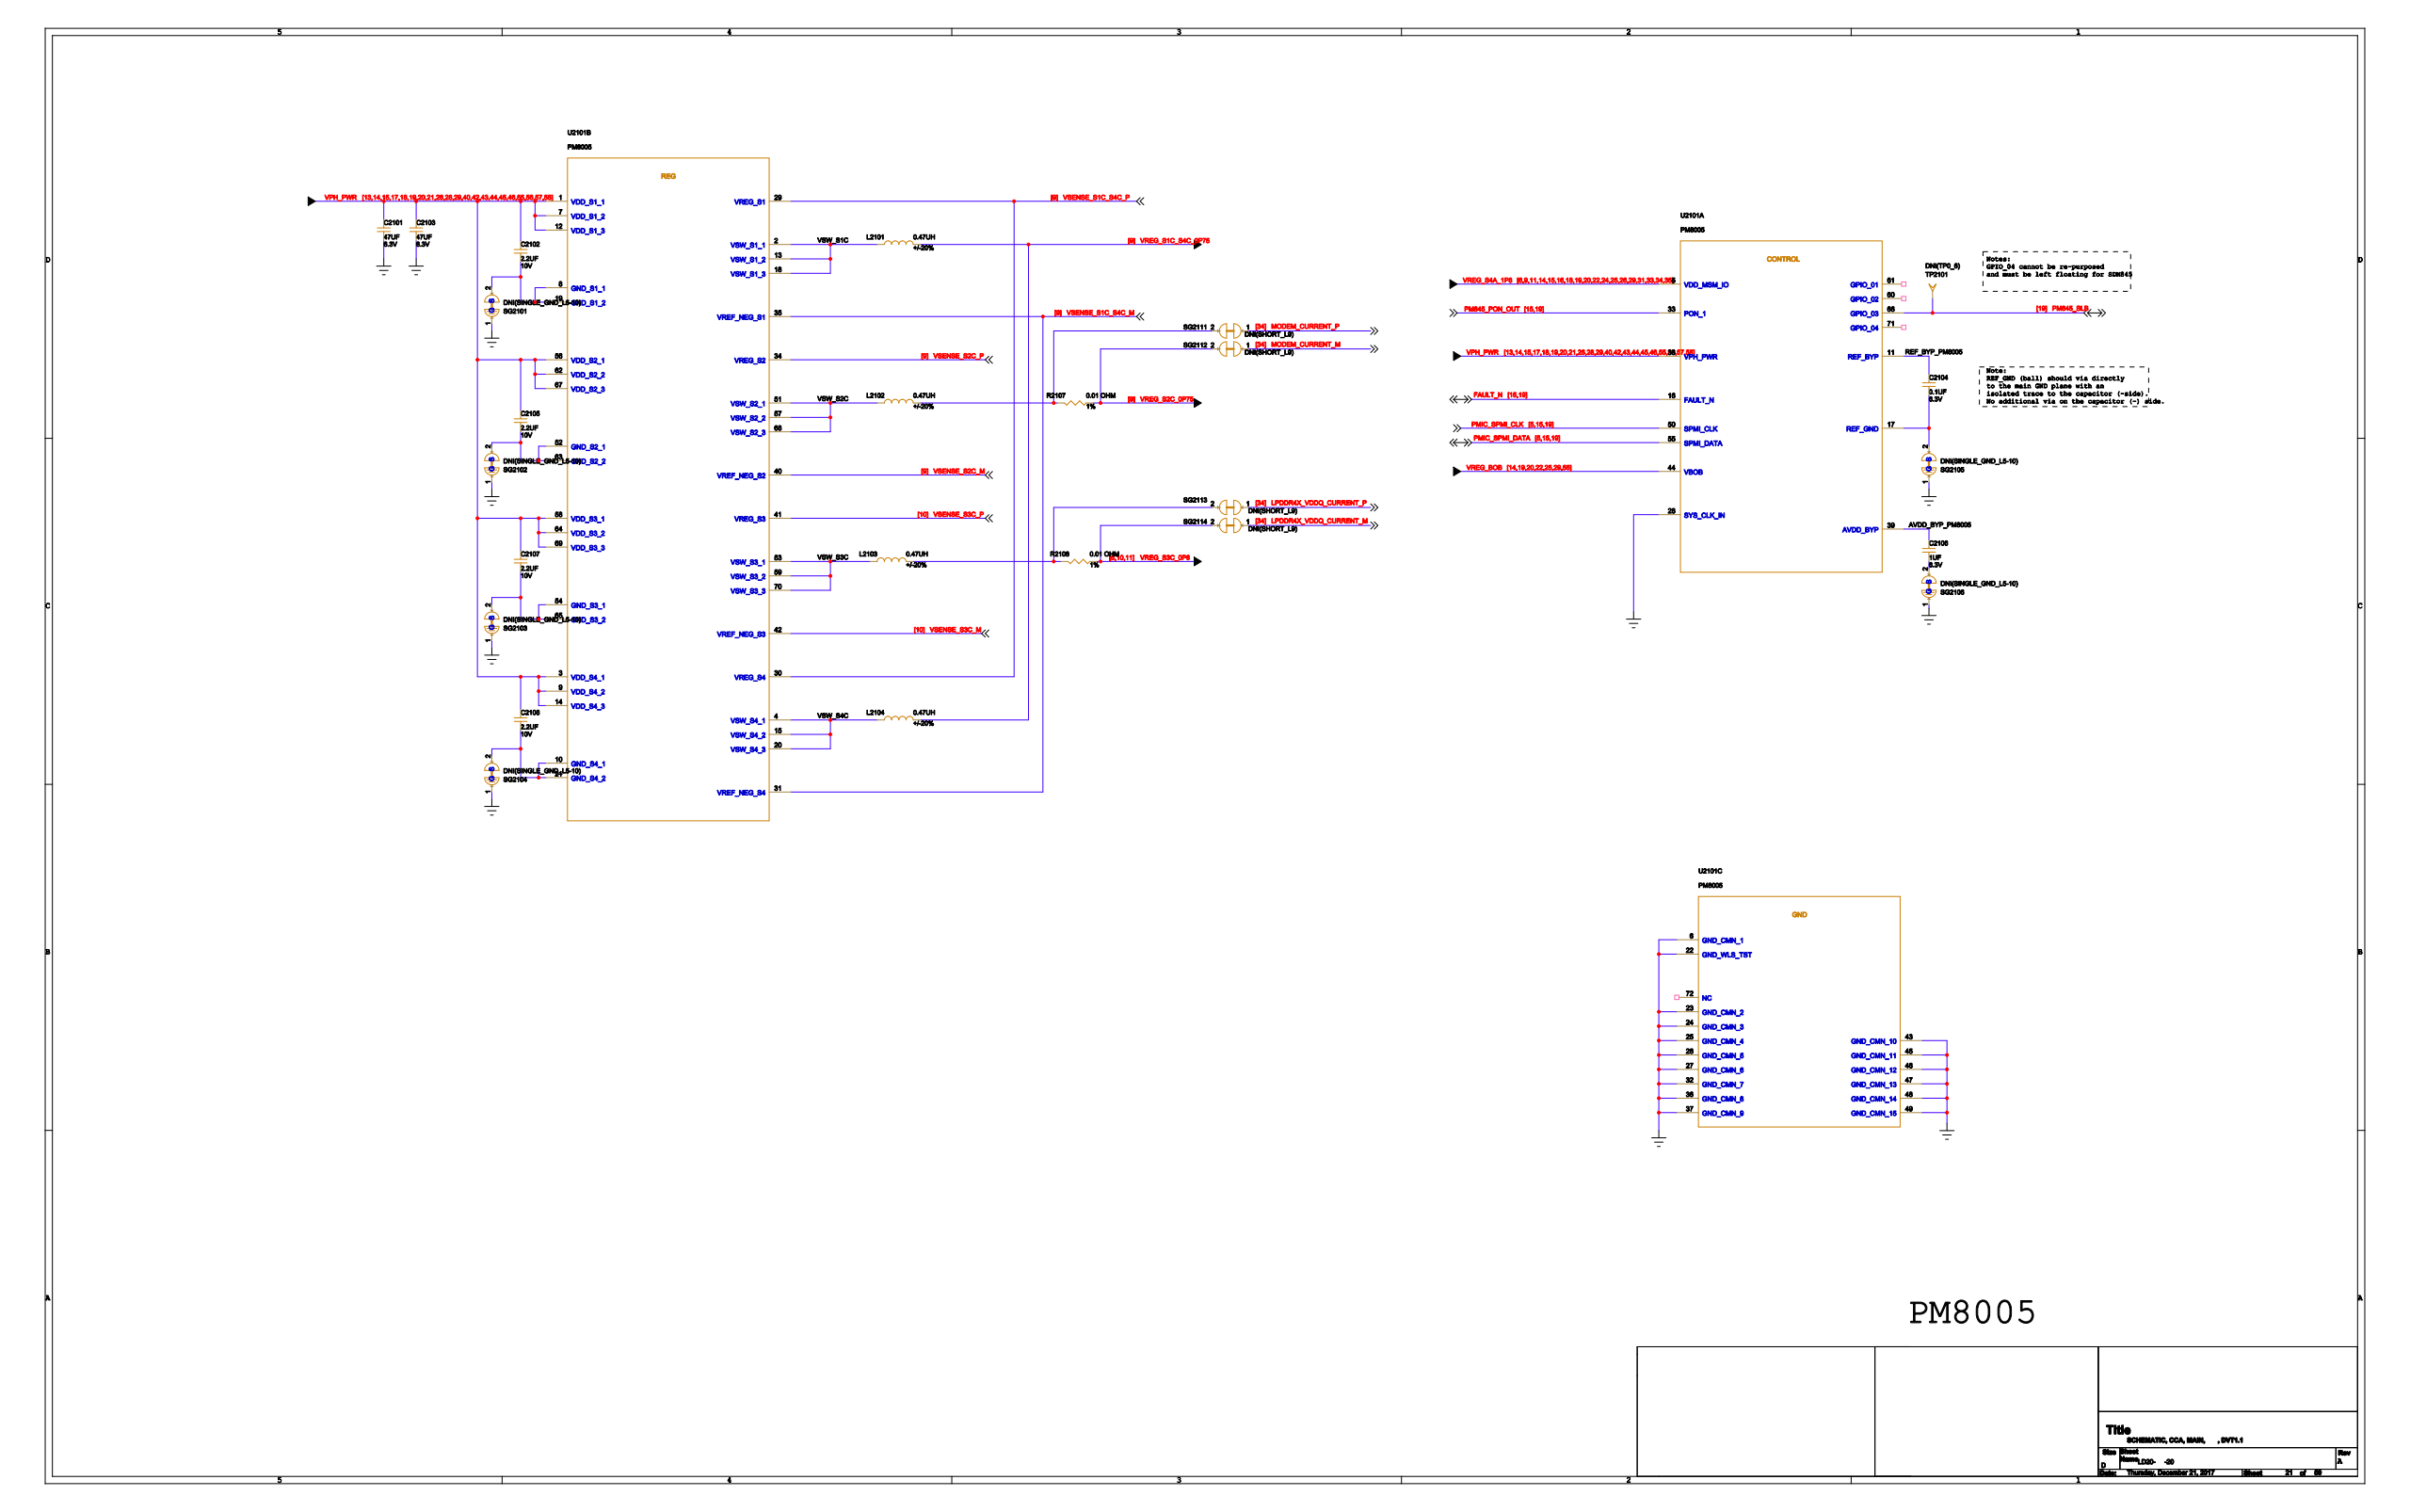Circuit board | Cadence Allegro | 1520 parts | 1149 nets | one sheet of the schematic
Parts on this sheet (reference | value | footprint):
C2101 | 47UF | 2P0603R
C2102 | 2.2UF | 2P0201R
C2103 | 47UF | 2P0603R
C2104 | 0.1UF | 2P0201R
C2105 | 2.2UF | 2P0201R
C2106 | 1UF | 2P0201R
C2107 | 2.2UF | 2P0201R
C2108 | 2.2UF | 2P0201R
L2101 | 0.47UH | 2PSM87X71NV2
L2102 | 0.47UH | 2PSM87X71NV2
L2103 | 0.47UH | 2PSM87X71NV2
L2104 | 0.47UH | 2PSM87X71NV2
R2107 | 0.01 OHM | 2P0603R
R2108 | 0.01 OHM | 2P0603R
SG2101 | DNI(SINGLE_GND_L5-10) | GND_L5-10
SG2102 | DNI(SINGLE_GND_L5-10) | GND_L5-10
SG2103 | DNI(SINGLE_GND_L5-10) | GND_L5-10
SG2104 | DNI(SINGLE_GND_L5-10) | GND_L5-10
SG2105 | DNI(SINGLE_GND_L5-10) | GND_L5-10
SG2106 | DNI(SINGLE_GND_L5-10) | GND_L5-10
SG2111 | DNI(SHORT_L9) | SHORT_L9_2REC08X12
SG2112 | DNI(SHORT_L9) | SHORT_L9_2REC08X12
SG2113 | DNI(SHORT_L9) | SHORT_L9_2REC08X12
SG2114 | DNI(SHORT_L9) | SHORT_L9_2REC08X12
TP2101 | DNI(TP0_6) | TP-0_6
U2101 | PM8005 | 72PGA137X113B138D45
Nets of these parts (net: part-pin ...):
GND: C2101-2 C2103-2 SG2101-1 SG2102-1 SG2103-1 SG2104-1 SG2105-1 SG2106-1 U2101-6 U2101-22 U2101-23 U2101-24 U2101-25 U2101-26 U2101-27 U2101-28 U2101-32 U2101-36 U2101-37 U2101-43 U2101-45 U2101-46 U2101-47 U2101-48 U2101-49
VREG_BOB: U2101-44
VREG_S4A_1P8: U2101-5
N34068033: C2102-2 SG2101-2 U2101-8 U2101-19
N34068049: C2105-2 SG2102-2 U2101-52 U2101-63
N34068057: C2107-2 SG2103-2 U2101-54 U2101-65
N34068063: C2108-2 SG2104-2 U2101-10 U2101-21
N34068437: C2104-2 SG2105-2 U2101-17
N34916750: C2106-2 SG2106-2
VPH_PWR: C2101-1 C2102-1 C2103-1 C2105-1 C2107-1 C2108-1 U2101-1 U2101-3 U2101-7 U2101-9 U2101-12 U2101-14 U2101-38 U2101-56 U2101-58 U2101-62 U2101-64 U2101-67 U2101-69
MODEM_CURRENT_P: SG2111-1
N34439854: L2102-2 R2107-1 SG2111-2
MODEM_CURRENT_M: SG2112-1
VREG_S2C_0P75: R2107-2 SG2112-2
LPDDR4X_VDDQ_CURRENT_P: SG2113-1
N34439887: L2103-2 R2108-1 SG2113-2
LPDDR4X_VDDQ_CURRENT_M: SG2114-1
VREG_S3C_0P6: R2108-2 SG2114-2
REF_BYP_PM8005: C2104-1 U2101-11
AVDD_BYP_PM8005: C2106-1 U2101-39
VREG_S1C_S4C_0P75: L2101-2 L2104-2
VSENSE_S2C_M: U2101-40
VSENSE_S1C_S4C_M: U2101-31 U2101-35
VSENSE_S2C_P: U2101-34
VSENSE_S1C_S4C_P: U2101-29 U2101-30
VSENSE_S3C_M: U2101-42
VSENSE_S3C_P: U2101-41
VSW_S1C: L2101-1 U2101-2 U2101-13 U2101-18
VSW_S2C: L2102-1 U2101-51 U2101-57 U2101-68
VSW_S3C: L2103-1 U2101-53 U2101-59 U2101-70
VSW_S4C: L2104-1 U2101-4 U2101-15 U2101-20
PMIC_SPMI_DATA: U2101-55
PMIC_SPMI_CLK: U2101-50
FAULT_N: U2101-16
PM845_PON_OUT: U2101-33
PM845_SLB: TP2101-1 U2101-66